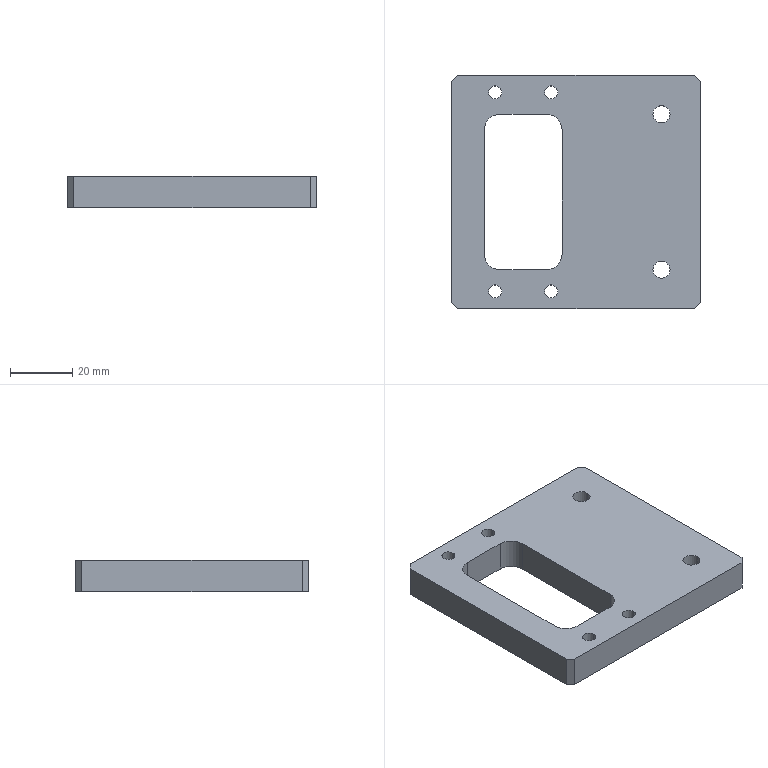Part | SolidWorks | features HoleWzd 2, Chamfer 1, Cut 1, Extrusion 1 | 1 solid | 36 faces | box 80 x 75 x 10 mm | volume 45981 mm3 | cylinder 20 | plane 16 | commonest cylinder face diameters 4.2 x8 10 x8 5.5 x4
STEP:
#1=CARTESIAN_POINT('',(-5.899,32.,5.));
#2=VERTEX_POINT('',#1);
#3=CARTESIAN_POINT('',(-10.099,32.,5.));
#4=VERTEX_POINT('',#3);
#5=CARTESIAN_POINT('',(-7.999,32.,5.));
#6=DIRECTION('',(0.,0.,-1.));
#7=DIRECTION('',(-1.,0.,0.));
#8=AXIS2_PLACEMENT_3D('',#5,#6,#7);
#9=CIRCLE('',#8,2.1);
#10=EDGE_CURVE('',#2,#4,#9,.T.);
#11=ORIENTED_EDGE('',*,*,#10,.F.);
#12=CARTESIAN_POINT('',(-5.899,32.,-5.));
#13=VERTEX_POINT('',#12);
#14=CARTESIAN_POINT('',(-5.899,32.,-5.));
#15=DIRECTION('',(0.,0.,-1.));
#16=VECTOR('',#15,1000.);
#17=LINE('',#14,#16);
#18=EDGE_CURVE('',#2,#13,#17,.T.);
#19=ORIENTED_EDGE('',*,*,#18,.T.);
#20=CARTESIAN_POINT('',(-10.099,32.,-5.));
#21=VERTEX_POINT('',#20);
#22=CARTESIAN_POINT('',(-7.999,32.,-5.));
#23=DIRECTION('',(0.,0.,-1.));
#24=DIRECTION('',(-1.,0.,0.));
#25=AXIS2_PLACEMENT_3D('',#22,#23,#24);
#26=CIRCLE('',#25,2.1);
#27=EDGE_CURVE('',#13,#21,#26,.T.);
#28=ORIENTED_EDGE('',*,*,#27,.T.);
#29=CARTESIAN_POINT('',(-10.099,32.,-5.));
#30=DIRECTION('',(0.,0.,-1.));
#31=VECTOR('',#30,1000.);
#32=LINE('',#29,#31);
#33=EDGE_CURVE('',#4,#21,#32,.T.);
#34=ORIENTED_EDGE('',*,*,#33,.F.);
#35=EDGE_LOOP('',(#11,#19,#28,#34));
#36=FACE_OUTER_BOUND('',#35,.T.);
#37=CARTESIAN_POINT('',(-7.999,32.,-5.));
#38=DIRECTION('',(0.,0.,-1.));
#39=DIRECTION('',(-1.,0.,0.));
#40=AXIS2_PLACEMENT_3D('',#37,#38,#39);
#41=CYLINDRICAL_SURFACE('',#40,2.1);
#42=ADVANCED_FACE('',(#36),#41,.F.);
#43=CARTESIAN_POINT('',(-23.899,32.,5.));
#44=VERTEX_POINT('',#43);
#45=CARTESIAN_POINT('',(-28.099,32.,5.));
#46=VERTEX_POINT('',#45);
#47=CARTESIAN_POINT('',(-25.999,32.,5.));
#48=DIRECTION('',(0.,0.,-1.));
#49=DIRECTION('',(-1.,0.,0.));
#50=AXIS2_PLACEMENT_3D('',#47,#48,#49);
#51=CIRCLE('',#50,2.1);
#52=EDGE_CURVE('',#44,#46,#51,.T.);
#53=ORIENTED_EDGE('',*,*,#52,.F.);
#54=CARTESIAN_POINT('',(-23.899,32.,-5.));
#55=VERTEX_POINT('',#54);
#56=CARTESIAN_POINT('',(-23.899,32.,-5.));
#57=DIRECTION('',(0.,0.,-1.));
#58=VECTOR('',#57,1000.);
#59=LINE('',#56,#58);
#60=EDGE_CURVE('',#44,#55,#59,.T.);
#61=ORIENTED_EDGE('',*,*,#60,.T.);
#62=CARTESIAN_POINT('',(-28.099,32.,-5.));
#63=VERTEX_POINT('',#62);
#64=CARTESIAN_POINT('',(-25.999,32.,-5.));
#65=DIRECTION('',(0.,0.,-1.));
#66=DIRECTION('',(-1.,0.,0.));
#67=AXIS2_PLACEMENT_3D('',#64,#65,#66);
#68=CIRCLE('',#67,2.1);
#69=EDGE_CURVE('',#55,#63,#68,.T.);
#70=ORIENTED_EDGE('',*,*,#69,.T.);
#71=CARTESIAN_POINT('',(-28.099,32.,-5.));
#72=DIRECTION('',(0.,0.,-1.));
#73=VECTOR('',#72,1000.);
#74=LINE('',#71,#73);
#75=EDGE_CURVE('',#46,#63,#74,.T.);
#76=ORIENTED_EDGE('',*,*,#75,.F.);
#77=EDGE_LOOP('',(#53,#61,#70,#76));
#78=FACE_OUTER_BOUND('',#77,.T.);
#79=CARTESIAN_POINT('',(-25.999,32.,-5.));
#80=DIRECTION('',(0.,0.,-1.));
#81=DIRECTION('',(-1.,0.,0.));
#82=AXIS2_PLACEMENT_3D('',#79,#80,#81);
#83=CYLINDRICAL_SURFACE('',#82,2.1);
#84=ADVANCED_FACE('',(#78),#83,.F.);
#85=CARTESIAN_POINT('',(-5.899,-32.,5.));
#86=VERTEX_POINT('',#85);
#87=CARTESIAN_POINT('',(-10.099,-32.,5.));
#88=VERTEX_POINT('',#87);
#89=CARTESIAN_POINT('',(-7.999,-32.,5.));
#90=DIRECTION('',(0.,0.,-1.));
#91=DIRECTION('',(-1.,0.,0.));
#92=AXIS2_PLACEMENT_3D('',#89,#90,#91);
#93=CIRCLE('',#92,2.1);
#94=EDGE_CURVE('',#86,#88,#93,.T.);
#95=ORIENTED_EDGE('',*,*,#94,.F.);
#96=CARTESIAN_POINT('',(-5.899,-32.,-5.));
#97=VERTEX_POINT('',#96);
#98=CARTESIAN_POINT('',(-5.899,-32.,-5.));
#99=DIRECTION('',(0.,0.,-1.));
#100=VECTOR('',#99,1000.);
#101=LINE('',#98,#100);
#102=EDGE_CURVE('',#86,#97,#101,.T.);
#103=ORIENTED_EDGE('',*,*,#102,.T.);
#104=CARTESIAN_POINT('',(-10.099,-32.,-5.));
#105=VERTEX_POINT('',#104);
#106=CARTESIAN_POINT('',(-7.999,-32.,-5.));
#107=DIRECTION('',(0.,0.,-1.));
#108=DIRECTION('',(-1.,0.,0.));
#109=AXIS2_PLACEMENT_3D('',#106,#107,#108);
#110=CIRCLE('',#109,2.1);
#111=EDGE_CURVE('',#97,#105,#110,.T.);
#112=ORIENTED_EDGE('',*,*,#111,.T.);
#113=CARTESIAN_POINT('',(-10.099,-32.,-5.));
#114=DIRECTION('',(0.,0.,-1.));
#115=VECTOR('',#114,1000.);
#116=LINE('',#113,#115);
#117=EDGE_CURVE('',#88,#105,#116,.T.);
#118=ORIENTED_EDGE('',*,*,#117,.F.);
#119=EDGE_LOOP('',(#95,#103,#112,#118));
#120=FACE_OUTER_BOUND('',#119,.T.);
#121=CARTESIAN_POINT('',(-7.999,-32.,-5.));
#122=DIRECTION('',(0.,0.,-1.));
#123=DIRECTION('',(-1.,0.,0.));
#124=AXIS2_PLACEMENT_3D('',#121,#122,#123);
#125=CYLINDRICAL_SURFACE('',#124,2.1);
#126=ADVANCED_FACE('',(#120),#125,.F.);
#127=CARTESIAN_POINT('',(-23.899,-32.,5.));
#128=VERTEX_POINT('',#127);
#129=CARTESIAN_POINT('',(-28.099,-32.,5.));
#130=VERTEX_POINT('',#129);
#131=CARTESIAN_POINT('',(-25.999,-32.,5.));
#132=DIRECTION('',(0.,0.,-1.));
#133=DIRECTION('',(-1.,0.,0.));
#134=AXIS2_PLACEMENT_3D('',#131,#132,#133);
#135=CIRCLE('',#134,2.1);
#136=EDGE_CURVE('',#128,#130,#135,.T.);
#137=ORIENTED_EDGE('',*,*,#136,.F.);
#138=CARTESIAN_POINT('',(-23.899,-32.,-5.));
#139=VERTEX_POINT('',#138);
#140=CARTESIAN_POINT('',(-23.899,-32.,-5.));
#141=DIRECTION('',(0.,0.,-1.));
#142=VECTOR('',#141,1000.);
#143=LINE('',#140,#142);
#144=EDGE_CURVE('',#128,#139,#143,.T.);
#145=ORIENTED_EDGE('',*,*,#144,.T.);
#146=CARTESIAN_POINT('',(-28.099,-32.,-5.));
#147=VERTEX_POINT('',#146);
#148=CARTESIAN_POINT('',(-25.999,-32.,-5.));
#149=DIRECTION('',(0.,0.,-1.));
#150=DIRECTION('',(-1.,0.,0.));
#151=AXIS2_PLACEMENT_3D('',#148,#149,#150);
#152=CIRCLE('',#151,2.1);
#153=EDGE_CURVE('',#139,#147,#152,.T.);
#154=ORIENTED_EDGE('',*,*,#153,.T.);
#155=CARTESIAN_POINT('',(-28.099,-32.,-5.));
#156=DIRECTION('',(0.,0.,-1.));
#157=VECTOR('',#156,1000.);
#158=LINE('',#155,#157);
#159=EDGE_CURVE('',#130,#147,#158,.T.);
#160=ORIENTED_EDGE('',*,*,#159,.F.);
#161=EDGE_LOOP('',(#137,#145,#154,#160));
#162=FACE_OUTER_BOUND('',#161,.T.);
#163=CARTESIAN_POINT('',(-25.999,-32.,-5.));
#164=DIRECTION('',(0.,0.,-1.));
#165=DIRECTION('',(-1.,0.,0.));
#166=AXIS2_PLACEMENT_3D('',#163,#164,#165);
#167=CYLINDRICAL_SURFACE('',#166,2.1);
#168=ADVANCED_FACE('',(#162),#167,.F.);
#169=CARTESIAN_POINT('',(32.5,25.,0.7));
#170=VERTEX_POINT('',#169);
#171=CARTESIAN_POINT('',(22.5,25.,0.7));
#172=VERTEX_POINT('',#171);
#173=CARTESIAN_POINT('',(27.5,25.,0.7));
#174=DIRECTION('',(0.,0.,-1.));
#175=DIRECTION('',(-1.,0.,0.));
#176=AXIS2_PLACEMENT_3D('',#173,#174,#175);
#177=CIRCLE('',#176,5.);
#178=EDGE_CURVE('',#170,#172,#177,.T.);
#179=ORIENTED_EDGE('',*,*,#178,.F.);
#180=CARTESIAN_POINT('',(32.5,25.,-5.));
#181=VERTEX_POINT('',#180);
#182=CARTESIAN_POINT('',(32.5,25.,-5.));
#183=DIRECTION('',(0.,0.,-1.));
#184=VECTOR('',#183,1000.);
#185=LINE('',#182,#184);
#186=EDGE_CURVE('',#170,#181,#185,.T.);
#187=ORIENTED_EDGE('',*,*,#186,.T.);
#188=CARTESIAN_POINT('',(22.5,25.,-5.));
#189=VERTEX_POINT('',#188);
#190=CARTESIAN_POINT('',(27.5,25.,-5.));
#191=DIRECTION('',(0.,0.,-1.));
#192=DIRECTION('',(-1.,0.,0.));
#193=AXIS2_PLACEMENT_3D('',#190,#191,#192);
#194=CIRCLE('',#193,5.);
#195=EDGE_CURVE('',#181,#189,#194,.T.);
#196=ORIENTED_EDGE('',*,*,#195,.T.);
#197=CARTESIAN_POINT('',(22.5,25.,-5.));
#198=DIRECTION('',(0.,0.,-1.));
#199=VECTOR('',#198,1000.);
#200=LINE('',#197,#199);
#201=EDGE_CURVE('',#172,#189,#200,.T.);
#202=ORIENTED_EDGE('',*,*,#201,.F.);
#203=EDGE_LOOP('',(#179,#187,#196,#202));
#204=FACE_OUTER_BOUND('',#203,.T.);
#205=CARTESIAN_POINT('',(27.5,25.,-5.));
#206=DIRECTION('',(0.,0.,-1.));
#207=DIRECTION('',(-1.,0.,0.));
#208=AXIS2_PLACEMENT_3D('',#205,#206,#207);
#209=CYLINDRICAL_SURFACE('',#208,5.);
#210=ADVANCED_FACE('',(#204),#209,.F.);
#211=CARTESIAN_POINT('',(30.25,25.,5.));
#212=VERTEX_POINT('',#211);
#213=CARTESIAN_POINT('',(24.75,25.,5.));
#214=VERTEX_POINT('',#213);
#215=CARTESIAN_POINT('',(27.5,25.,5.));
#216=DIRECTION('',(0.,0.,-1.));
#217=DIRECTION('',(-1.,0.,0.));
#218=AXIS2_PLACEMENT_3D('',#215,#216,#217);
#219=CIRCLE('',#218,2.75);
#220=EDGE_CURVE('',#212,#214,#219,.T.);
#221=ORIENTED_EDGE('',*,*,#220,.F.);
#222=CARTESIAN_POINT('',(30.25,25.,0.7));
#223=VERTEX_POINT('',#222);
#224=CARTESIAN_POINT('',(30.25,25.,-5.));
#225=DIRECTION('',(0.,0.,-1.));
#226=VECTOR('',#225,1000.);
#227=LINE('',#224,#226);
#228=EDGE_CURVE('',#212,#223,#227,.T.);
#229=ORIENTED_EDGE('',*,*,#228,.T.);
#230=CARTESIAN_POINT('',(24.75,25.,0.7));
#231=VERTEX_POINT('',#230);
#232=CARTESIAN_POINT('',(27.5,25.,0.7));
#233=DIRECTION('',(0.,0.,-1.));
#234=DIRECTION('',(-1.,0.,0.));
#235=AXIS2_PLACEMENT_3D('',#232,#233,#234);
#236=CIRCLE('',#235,2.75);
#237=EDGE_CURVE('',#223,#231,#236,.T.);
#238=ORIENTED_EDGE('',*,*,#237,.T.);
#239=CARTESIAN_POINT('',(24.75,25.,-5.));
#240=DIRECTION('',(0.,0.,-1.));
#241=VECTOR('',#240,1000.);
#242=LINE('',#239,#241);
#243=EDGE_CURVE('',#214,#231,#242,.T.);
#244=ORIENTED_EDGE('',*,*,#243,.F.);
#245=EDGE_LOOP('',(#221,#229,#238,#244));
#246=FACE_OUTER_BOUND('',#245,.T.);
#247=CARTESIAN_POINT('',(27.5,25.,-5.));
#248=DIRECTION('',(0.,0.,-1.));
#249=DIRECTION('',(-1.,0.,0.));
#250=AXIS2_PLACEMENT_3D('',#247,#248,#249);
#251=CYLINDRICAL_SURFACE('',#250,2.75);
#252=ADVANCED_FACE('',(#246),#251,.F.);
#253=CARTESIAN_POINT('',(32.5,-25.,0.7));
#254=VERTEX_POINT('',#253);
#255=CARTESIAN_POINT('',(22.5,-25.,0.7));
#256=VERTEX_POINT('',#255);
#257=CARTESIAN_POINT('',(27.5,-25.,0.7));
#258=DIRECTION('',(0.,0.,-1.));
#259=DIRECTION('',(-1.,0.,0.));
#260=AXIS2_PLACEMENT_3D('',#257,#258,#259);
#261=CIRCLE('',#260,5.);
#262=EDGE_CURVE('',#254,#256,#261,.T.);
#263=ORIENTED_EDGE('',*,*,#262,.F.);
#264=CARTESIAN_POINT('',(32.5,-25.,-5.));
#265=VERTEX_POINT('',#264);
#266=CARTESIAN_POINT('',(32.5,-25.,-5.));
#267=DIRECTION('',(0.,0.,-1.));
#268=VECTOR('',#267,1000.);
#269=LINE('',#266,#268);
#270=EDGE_CURVE('',#254,#265,#269,.T.);
#271=ORIENTED_EDGE('',*,*,#270,.T.);
#272=CARTESIAN_POINT('',(22.5,-25.,-5.));
#273=VERTEX_POINT('',#272);
#274=CARTESIAN_POINT('',(27.5,-25.,-5.));
#275=DIRECTION('',(0.,0.,-1.));
#276=DIRECTION('',(-1.,0.,0.));
#277=AXIS2_PLACEMENT_3D('',#274,#275,#276);
#278=CIRCLE('',#277,5.);
#279=EDGE_CURVE('',#265,#273,#278,.T.);
#280=ORIENTED_EDGE('',*,*,#279,.T.);
#281=CARTESIAN_POINT('',(22.5,-25.,-5.));
#282=DIRECTION('',(0.,0.,-1.));
#283=VECTOR('',#282,1000.);
#284=LINE('',#281,#283);
#285=EDGE_CURVE('',#256,#273,#284,.T.);
#286=ORIENTED_EDGE('',*,*,#285,.F.);
#287=EDGE_LOOP('',(#263,#271,#280,#286));
#288=FACE_OUTER_BOUND('',#287,.T.);
#289=CARTESIAN_POINT('',(27.5,-25.,-5.));
#290=DIRECTION('',(0.,0.,-1.));
#291=DIRECTION('',(-1.,0.,0.));
#292=AXIS2_PLACEMENT_3D('',#289,#290,#291);
#293=CYLINDRICAL_SURFACE('',#292,5.);
#294=ADVANCED_FACE('',(#288),#293,.F.);
#295=CARTESIAN_POINT('',(30.25,-25.,5.));
#296=VERTEX_POINT('',#295);
#297=CARTESIAN_POINT('',(24.75,-25.,5.));
#298=VERTEX_POINT('',#297);
#299=CARTESIAN_POINT('',(27.5,-25.,5.));
#300=DIRECTION('',(0.,0.,-1.));
#301=DIRECTION('',(-1.,0.,0.));
#302=AXIS2_PLACEMENT_3D('',#299,#300,#301);
#303=CIRCLE('',#302,2.75);
#304=EDGE_CURVE('',#296,#298,#303,.T.);
#305=ORIENTED_EDGE('',*,*,#304,.F.);
#306=CARTESIAN_POINT('',(30.25,-25.,0.7));
#307=VERTEX_POINT('',#306);
#308=CARTESIAN_POINT('',(30.25,-25.,-5.));
#309=DIRECTION('',(0.,0.,-1.));
#310=VECTOR('',#309,1000.);
#311=LINE('',#308,#310);
#312=EDGE_CURVE('',#296,#307,#311,.T.);
#313=ORIENTED_EDGE('',*,*,#312,.T.);
#314=CARTESIAN_POINT('',(24.75,-25.,0.7));
#315=VERTEX_POINT('',#314);
#316=CARTESIAN_POINT('',(27.5,-25.,0.7));
#317=DIRECTION('',(0.,0.,-1.));
#318=DIRECTION('',(-1.,0.,0.));
#319=AXIS2_PLACEMENT_3D('',#316,#317,#318);
#320=CIRCLE('',#319,2.75);
#321=EDGE_CURVE('',#307,#315,#320,.T.);
#322=ORIENTED_EDGE('',*,*,#321,.T.);
#323=CARTESIAN_POINT('',(24.75,-25.,-5.));
#324=DIRECTION('',(0.,0.,-1.));
#325=VECTOR('',#324,1000.);
#326=LINE('',#323,#325);
#327=EDGE_CURVE('',#298,#315,#326,.T.);
#328=ORIENTED_EDGE('',*,*,#327,.F.);
#329=EDGE_LOOP('',(#305,#313,#322,#328));
#330=FACE_OUTER_BOUND('',#329,.T.);
#331=CARTESIAN_POINT('',(27.5,-25.,-5.));
#332=DIRECTION('',(0.,0.,-1.));
#333=DIRECTION('',(-1.,0.,0.));
#334=AXIS2_PLACEMENT_3D('',#331,#332,#333);
#335=CYLINDRICAL_SURFACE('',#334,2.75);
#336=ADVANCED_FACE('',(#330),#335,.F.);
#337=CARTESIAN_POINT('',(40.,-35.5,5.));
#338=VERTEX_POINT('',#337);
#339=CARTESIAN_POINT('',(40.,35.5,5.));
#340=VERTEX_POINT('',#339);
#341=CARTESIAN_POINT('',(40.,-37.5,5.));
#342=DIRECTION('',(0.,1.,0.));
#343=VECTOR('',#342,1000.);
#344=LINE('',#341,#343);
#345=EDGE_CURVE('',#338,#340,#344,.T.);
#346=ORIENTED_EDGE('',*,*,#345,.F.);
#347=CARTESIAN_POINT('',(40.,-35.5,-5.));
#348=VERTEX_POINT('',#347);
#349=CARTESIAN_POINT('',(40.,-35.5,5.));
#350=DIRECTION('',(0.,0.,-1.));
#351=VECTOR('',#350,1000.);
#352=LINE('',#349,#351);
#353=EDGE_CURVE('',#338,#348,#352,.T.);
#354=ORIENTED_EDGE('',*,*,#353,.T.);
#355=CARTESIAN_POINT('',(40.,35.5,-5.));
#356=VERTEX_POINT('',#355);
#357=CARTESIAN_POINT('',(40.,-37.5,-5.));
#358=DIRECTION('',(0.,1.,0.));
#359=VECTOR('',#358,1000.);
#360=LINE('',#357,#359);
#361=EDGE_CURVE('',#348,#356,#360,.T.);
#362=ORIENTED_EDGE('',*,*,#361,.T.);
#363=CARTESIAN_POINT('',(40.,35.5,5.));
#364=DIRECTION('',(0.,0.,1.));
#365=VECTOR('',#364,1000.);
#366=LINE('',#363,#365);
#367=EDGE_CURVE('',#356,#340,#366,.T.);
#368=ORIENTED_EDGE('',*,*,#367,.T.);
#369=EDGE_LOOP('',(#346,#354,#362,#368));
#370=FACE_OUTER_BOUND('',#369,.T.);
#371=CARTESIAN_POINT('',(40.,-37.5,5.));
#372=DIRECTION('',(-1.,0.,0.));
#373=DIRECTION('',(0.,0.,1.));
#374=AXIS2_PLACEMENT_3D('',#371,#372,#373);
#375=PLANE('',#374);
#376=ADVANCED_FACE('',(#370),#375,.F.);
#377=CARTESIAN_POINT('',(38.,37.5,-5.));
#378=VERTEX_POINT('',#377);
#379=CARTESIAN_POINT('',(-38.,37.5,-5.));
#380=VERTEX_POINT('',#379);
#381=CARTESIAN_POINT('',(-40.,37.5,-5.));
#382=DIRECTION('',(-1.,0.,0.));
#383=VECTOR('',#382,1000.);
#384=LINE('',#381,#383);
#385=EDGE_CURVE('',#378,#380,#384,.T.);
#386=ORIENTED_EDGE('',*,*,#385,.T.);
#387=CARTESIAN_POINT('',(-38.,37.5,5.));
#388=VERTEX_POINT('',#387);
#389=CARTESIAN_POINT('',(-38.,37.5,5.));
#390=DIRECTION('',(0.,0.,1.));
#391=VECTOR('',#390,1000.);
#392=LINE('',#389,#391);
#393=EDGE_CURVE('',#380,#388,#392,.T.);
#394=ORIENTED_EDGE('',*,*,#393,.T.);
#395=CARTESIAN_POINT('',(38.,37.5,5.));
#396=VERTEX_POINT('',#395);
#397=CARTESIAN_POINT('',(-40.,37.5,5.));
#398=DIRECTION('',(-1.,0.,0.));
#399=VECTOR('',#398,1000.);
#400=LINE('',#397,#399);
#401=EDGE_CURVE('',#396,#388,#400,.T.);
#402=ORIENTED_EDGE('',*,*,#401,.F.);
#403=CARTESIAN_POINT('',(38.,37.5,5.));
#404=DIRECTION('',(0.,0.,-1.));
#405=VECTOR('',#404,1000.);
#406=LINE('',#403,#405);
#407=EDGE_CURVE('',#396,#378,#406,.T.);
#408=ORIENTED_EDGE('',*,*,#407,.T.);
#409=EDGE_LOOP('',(#386,#394,#402,#408));
#410=FACE_OUTER_BOUND('',#409,.T.);
#411=CARTESIAN_POINT('',(-40.,37.5,5.));
#412=DIRECTION('',(0.,-1.,0.));
#413=DIRECTION('',(0.,0.,-1.));
#414=AXIS2_PLACEMENT_3D('',#411,#412,#413);
#415=PLANE('',#414);
#416=ADVANCED_FACE('',(#410),#415,.F.);
#417=CARTESIAN_POINT('',(-40.,35.5,-5.));
#418=VERTEX_POINT('',#417);
#419=CARTESIAN_POINT('',(-40.,-35.5,-5.));
#420=VERTEX_POINT('',#419);
#421=CARTESIAN_POINT('',(-40.,-37.5,-5.));
#422=DIRECTION('',(0.,-1.,0.));
#423=VECTOR('',#422,1000.);
#424=LINE('',#421,#423);
#425=EDGE_CURVE('',#418,#420,#424,.T.);
#426=ORIENTED_EDGE('',*,*,#425,.T.);
#427=CARTESIAN_POINT('',(-40.,-35.5,5.));
#428=VERTEX_POINT('',#427);
#429=CARTESIAN_POINT('',(-40.,-35.5,5.));
#430=DIRECTION('',(0.,0.,1.));
#431=VECTOR('',#430,1000.);
#432=LINE('',#429,#431);
#433=EDGE_CURVE('',#420,#428,#432,.T.);
#434=ORIENTED_EDGE('',*,*,#433,.T.);
#435=CARTESIAN_POINT('',(-40.,35.5,5.));
#436=VERTEX_POINT('',#435);
#437=CARTESIAN_POINT('',(-40.,-37.5,5.));
#438=DIRECTION('',(0.,-1.,0.));
#439=VECTOR('',#438,1000.);
#440=LINE('',#437,#439);
#441=EDGE_CURVE('',#436,#428,#440,.T.);
#442=ORIENTED_EDGE('',*,*,#441,.F.);
#443=CARTESIAN_POINT('',(-40.,35.5,5.));
#444=DIRECTION('',(0.,0.,-1.));
#445=VECTOR('',#444,1000.);
#446=LINE('',#443,#445);
#447=EDGE_CURVE('',#436,#418,#446,.T.);
#448=ORIENTED_EDGE('',*,*,#447,.T.);
#449=EDGE_LOOP('',(#426,#434,#442,#448));
#450=FACE_OUTER_BOUND('',#449,.T.);
#451=CARTESIAN_POINT('',(-40.,-37.5,5.));
#452=DIRECTION('',(1.,0.,0.));
#453=DIRECTION('',(0.,0.,-1.));
#454=AXIS2_PLACEMENT_3D('',#451,#452,#453);
#455=PLANE('',#454);
#456=ADVANCED_FACE('',(#450),#455,.F.);
#457=CARTESIAN_POINT('',(-38.,-37.5,-5.));
#458=VERTEX_POINT('',#457);
#459=CARTESIAN_POINT('',(38.,-37.5,-5.));
#460=VERTEX_POINT('',#459);
#461=CARTESIAN_POINT('',(-40.,-37.5,-5.));
#462=DIRECTION('',(1.,0.,0.));
#463=VECTOR('',#462,1000.);
#464=LINE('',#461,#463);
#465=EDGE_CURVE('',#458,#460,#464,.T.);
#466=ORIENTED_EDGE('',*,*,#465,.T.);
#467=CARTESIAN_POINT('',(38.,-37.5,5.));
#468=VERTEX_POINT('',#467);
#469=CARTESIAN_POINT('',(38.,-37.5,5.));
#470=DIRECTION('',(0.,0.,1.));
#471=VECTOR('',#470,1000.);
#472=LINE('',#469,#471);
#473=EDGE_CURVE('',#460,#468,#472,.T.);
#474=ORIENTED_EDGE('',*,*,#473,.T.);
#475=CARTESIAN_POINT('',(-38.,-37.5,5.));
#476=VERTEX_POINT('',#475);
#477=CARTESIAN_POINT('',(-40.,-37.5,5.));
#478=DIRECTION('',(1.,0.,0.));
#479=VECTOR('',#478,1000.);
#480=LINE('',#477,#479);
#481=EDGE_CURVE('',#476,#468,#480,.T.);
#482=ORIENTED_EDGE('',*,*,#481,.F.);
#483=CARTESIAN_POINT('',(-38.,-37.5,5.));
#484=DIRECTION('',(0.,0.,-1.));
#485=VECTOR('',#484,1000.);
#486=LINE('',#483,#485);
#487=EDGE_CURVE('',#476,#458,#486,.T.);
#488=ORIENTED_EDGE('',*,*,#487,.T.);
#489=EDGE_LOOP('',(#466,#474,#482,#488));
#490=FACE_OUTER_BOUND('',#489,.T.);
#491=CARTESIAN_POINT('',(-40.,-37.5,5.));
#492=DIRECTION('',(0.,1.,0.));
#493=DIRECTION('',(0.,0.,1.));
#494=AXIS2_PLACEMENT_3D('',#491,#492,#493);
#495=PLANE('',#494);
#496=ADVANCED_FACE('',(#490),#495,.F.);
#497=CARTESIAN_POINT('',(-9.499,-25.,5.));
#498=VERTEX_POINT('',#497);
#499=CARTESIAN_POINT('',(-24.499,-25.,5.));
#500=VERTEX_POINT('',#499);
#501=CARTESIAN_POINT('',(-9.499,-25.,5.));
#502=DIRECTION('',(-1.,0.,0.));
#503=VECTOR('',#502,1000.);
#504=LINE('',#501,#503);
#505=EDGE_CURVE('',#498,#500,#504,.T.);
#506=ORIENTED_EDGE('',*,*,#505,.T.);
#507=CARTESIAN_POINT('',(-29.499,-20.,5.));
#508=VERTEX_POINT('',#507);
#509=CARTESIAN_POINT('',(-24.499,-20.,5.));
#510=DIRECTION('',(0.,0.,-1.));
#511=DIRECTION('',(-1.,0.,0.));
#512=AXIS2_PLACEMENT_3D('',#509,#510,#511);
#513=CIRCLE('',#512,5.);
#514=EDGE_CURVE('',#500,#508,#513,.T.);
#515=ORIENTED_EDGE('',*,*,#514,.T.);
#516=CARTESIAN_POINT('',(-29.499,20.,5.));
#517=VERTEX_POINT('',#516);
#518=CARTESIAN_POINT('',(-29.499,-20.,5.));
#519=DIRECTION('',(0.,1.,0.));
#520=VECTOR('',#519,1000.);
#521=LINE('',#518,#520);
#522=EDGE_CURVE('',#508,#517,#521,.T.);
#523=ORIENTED_EDGE('',*,*,#522,.T.);
#524=CARTESIAN_POINT('',(-24.499,25.,5.));
#525=VERTEX_POINT('',#524);
#526=CARTESIAN_POINT('',(-24.499,20.,5.));
#527=DIRECTION('',(0.,0.,-1.));
#528=DIRECTION('',(1.,0.,0.));
#529=AXIS2_PLACEMENT_3D('',#526,#527,#528);
#530=CIRCLE('',#529,5.);
#531=EDGE_CURVE('',#517,#525,#530,.T.);
#532=ORIENTED_EDGE('',*,*,#531,.T.);
#533=CARTESIAN_POINT('',(-9.499,25.,5.));
#534=VERTEX_POINT('',#533);
#535=CARTESIAN_POINT('',(-9.499,25.,5.));
#536=DIRECTION('',(1.,0.,0.));
#537=VECTOR('',#536,1000.);
#538=LINE('',#535,#537);
#539=EDGE_CURVE('',#525,#534,#538,.T.);
#540=ORIENTED_EDGE('',*,*,#539,.T.);
#541=CARTESIAN_POINT('',(-4.499,20.,5.));
#542=VERTEX_POINT('',#541);
#543=CARTESIAN_POINT('',(-9.499,20.,5.));
#544=DIRECTION('',(0.,0.,-1.));
#545=DIRECTION('',(1.,0.,0.));
#546=AXIS2_PLACEMENT_3D('',#543,#544,#545);
#547=CIRCLE('',#546,5.);
#548=EDGE_CURVE('',#534,#542,#547,.T.);
#549=ORIENTED_EDGE('',*,*,#548,.T.);
#550=CARTESIAN_POINT('',(-4.499,-20.,5.));
#551=VERTEX_POINT('',#550);
#552=CARTESIAN_POINT('',(-4.499,-20.,5.));
#553=DIRECTION('',(0.,-1.,0.));
#554=VECTOR('',#553,1000.);
#555=LINE('',#552,#554);
#556=EDGE_CURVE('',#542,#551,#555,.T.);
#557=ORIENTED_EDGE('',*,*,#556,.T.);
#558=CARTESIAN_POINT('',(-9.499,-20.,5.));
#559=DIRECTION('',(0.,0.,-1.));
#560=DIRECTION('',(1.,0.,0.));
#561=AXIS2_PLACEMENT_3D('',#558,#559,#560);
#562=CIRCLE('',#561,5.);
#563=EDGE_CURVE('',#551,#498,#562,.T.);
#564=ORIENTED_EDGE('',*,*,#563,.T.);
#565=EDGE_LOOP('',(#506,#515,#523,#532,#540,#549,#557,#564));
#566=FACE_BOUND('',#565,.T.);
#567=CARTESIAN_POINT('',(-7.999,32.,5.));
#568=DIRECTION('',(0.,0.,-1.));
#569=DIRECTION('',(-1.,0.,0.));
#570=AXIS2_PLACEMENT_3D('',#567,#568,#569);
#571=CIRCLE('',#570,2.1);
#572=EDGE_CURVE('',#4,#2,#571,.T.);
#573=ORIENTED_EDGE('',*,*,#572,.T.);
#574=ORIENTED_EDGE('',*,*,#10,.T.);
#575=EDGE_LOOP('',(#573,#574));
#576=FACE_BOUND('',#575,.T.);
#577=CARTESIAN_POINT('',(-25.999,32.,5.));
#578=DIRECTION('',(0.,0.,-1.));
#579=DIRECTION('',(-1.,0.,0.));
#580=AXIS2_PLACEMENT_3D('',#577,#578,#579);
#581=CIRCLE('',#580,2.1);
#582=EDGE_CURVE('',#46,#44,#581,.T.);
#583=ORIENTED_EDGE('',*,*,#582,.T.);
#584=ORIENTED_EDGE('',*,*,#52,.T.);
#585=EDGE_LOOP('',(#583,#584));
#586=FACE_BOUND('',#585,.T.);
#587=CARTESIAN_POINT('',(-7.999,-32.,5.));
#588=DIRECTION('',(0.,0.,-1.));
#589=DIRECTION('',(-1.,0.,0.));
#590=AXIS2_PLACEMENT_3D('',#587,#588,#589);
#591=CIRCLE('',#590,2.1);
#592=EDGE_CURVE('',#88,#86,#591,.T.);
#593=ORIENTED_EDGE('',*,*,#592,.T.);
#594=ORIENTED_EDGE('',*,*,#94,.T.);
#595=EDGE_LOOP('',(#593,#594));
#596=FACE_BOUND('',#595,.T.);
#597=CARTESIAN_POINT('',(-25.999,-32.,5.));
#598=DIRECTION('',(0.,0.,-1.));
#599=DIRECTION('',(-1.,0.,0.));
#600=AXIS2_PLACEMENT_3D('',#597,#598,#599);
#601=CIRCLE('',#600,2.1);
#602=EDGE_CURVE('',#130,#128,#601,.T.);
#603=ORIENTED_EDGE('',*,*,#602,.T.);
#604=ORIENTED_EDGE('',*,*,#136,.T.);
#605=EDGE_LOOP('',(#603,#604));
#606=FACE_BOUND('',#605,.T.);
#607=CARTESIAN_POINT('',(27.5,25.,5.));
#608=DIRECTION('',(0.,0.,-1.));
#609=DIRECTION('',(-1.,0.,0.));
#610=AXIS2_PLACEMENT_3D('',#607,#608,#609);
#611=CIRCLE('',#610,2.75);
#612=EDGE_CURVE('',#214,#212,#611,.T.);
#613=ORIENTED_EDGE('',*,*,#612,.T.);
#614=ORIENTED_EDGE('',*,*,#220,.T.);
#615=EDGE_LOOP('',(#613,#614));
#616=FACE_BOUND('',#615,.T.);
#617=CARTESIAN_POINT('',(27.5,-25.,5.));
#618=DIRECTION('',(0.,0.,-1.));
#619=DIRECTION('',(-1.,0.,0.));
#620=AXIS2_PLACEMENT_3D('',#617,#618,#619);
#621=CIRCLE('',#620,2.75);
#622=EDGE_CURVE('',#298,#296,#621,.T.);
#623=ORIENTED_EDGE('',*,*,#622,.T.);
#624=ORIENTED_EDGE('',*,*,#304,.T.);
#625=EDGE_LOOP('',(#623,#624));
#626=FACE_BOUND('',#625,.T.);
#627=ORIENTED_EDGE('',*,*,#481,.T.);
#628=CARTESIAN_POINT('',(40.,-35.5,5.));
#629=DIRECTION('',(0.7071,0.7071,0.));
#630=VECTOR('',#629,1000.);
#631=LINE('',#628,#630);
#632=EDGE_CURVE('',#468,#338,#631,.T.);
#633=ORIENTED_EDGE('',*,*,#632,.T.);
#634=ORIENTED_EDGE('',*,*,#345,.T.);
#635=CARTESIAN_POINT('',(38.,37.5,5.));
#636=DIRECTION('',(-0.7071,0.7071,0.));
#637=VECTOR('',#636,1000.);
#638=LINE('',#635,#637);
#639=EDGE_CURVE('',#340,#396,#638,.T.);
#640=ORIENTED_EDGE('',*,*,#639,.T.);
#641=ORIENTED_EDGE('',*,*,#401,.T.);
#642=CARTESIAN_POINT('',(-40.,35.5,5.));
#643=DIRECTION('',(-0.7071,-0.7071,0.));
#644=VECTOR('',#643,1000.);
#645=LINE('',#642,#644);
#646=EDGE_CURVE('',#388,#436,#645,.T.);
#647=ORIENTED_EDGE('',*,*,#646,.T.);
#648=ORIENTED_EDGE('',*,*,#441,.T.);
#649=CARTESIAN_POINT('',(-38.,-37.5,5.));
#650=DIRECTION('',(0.7071,-0.7071,0.));
#651=VECTOR('',#650,1000.);
#652=LINE('',#649,#651);
#653=EDGE_CURVE('',#428,#476,#652,.T.);
#654=ORIENTED_EDGE('',*,*,#653,.T.);
#655=EDGE_LOOP('',(#627,#633,#634,#640,#641,#647,#648,#654));
#656=FACE_OUTER_BOUND('',#655,.T.);
#657=CARTESIAN_POINT('',(0.,0.,5.));
#658=DIRECTION('',(0.,0.,-1.));
#659=DIRECTION('',(-1.,0.,0.));
#660=AXIS2_PLACEMENT_3D('',#657,#658,#659);
#661=PLANE('',#660);
#662=ADVANCED_FACE('',(#566,#576,#586,#596,#606,#616,#626,#656),#661,.F.);
#663=CARTESIAN_POINT('',(-24.499,-25.,-5.));
#664=VERTEX_POINT('',#663);
#665=CARTESIAN_POINT('',(-29.499,-20.,-5.));
#666=VERTEX_POINT('',#665);
#667=CARTESIAN_POINT('',(-24.499,-20.,-5.));
#668=DIRECTION('',(0.,0.,-1.));
#669=DIRECTION('',(-1.,0.,0.));
#670=AXIS2_PLACEMENT_3D('',#667,#668,#669);
#671=CIRCLE('',#670,5.);
#672=EDGE_CURVE('',#664,#666,#671,.T.);
#673=ORIENTED_EDGE('',*,*,#672,.F.);
#674=CARTESIAN_POINT('',(-9.499,-25.,-5.));
#675=VERTEX_POINT('',#674);
#676=CARTESIAN_POINT('',(-9.499,-25.,-5.));
#677=DIRECTION('',(-1.,0.,0.));
#678=VECTOR('',#677,1000.);
#679=LINE('',#676,#678);
#680=EDGE_CURVE('',#675,#664,#679,.T.);
#681=ORIENTED_EDGE('',*,*,#680,.F.);
#682=CARTESIAN_POINT('',(-4.499,-20.,-5.));
#683=VERTEX_POINT('',#682);
#684=CARTESIAN_POINT('',(-9.499,-20.,-5.));
#685=DIRECTION('',(0.,0.,-1.));
#686=DIRECTION('',(1.,0.,0.));
#687=AXIS2_PLACEMENT_3D('',#684,#685,#686);
#688=CIRCLE('',#687,5.);
#689=EDGE_CURVE('',#683,#675,#688,.T.);
#690=ORIENTED_EDGE('',*,*,#689,.F.);
#691=CARTESIAN_POINT('',(-4.499,20.,-5.));
#692=VERTEX_POINT('',#691);
#693=CARTESIAN_POINT('',(-4.499,-20.,-5.));
#694=DIRECTION('',(0.,-1.,0.));
#695=VECTOR('',#694,1000.);
#696=LINE('',#693,#695);
#697=EDGE_CURVE('',#692,#683,#696,.T.);
#698=ORIENTED_EDGE('',*,*,#697,.F.);
#699=CARTESIAN_POINT('',(-9.499,25.,-5.));
#700=VERTEX_POINT('',#699);
#701=CARTESIAN_POINT('',(-9.499,20.,-5.));
#702=DIRECTION('',(0.,0.,-1.));
#703=DIRECTION('',(1.,0.,0.));
#704=AXIS2_PLACEMENT_3D('',#701,#702,#703);
#705=CIRCLE('',#704,5.);
#706=EDGE_CURVE('',#700,#692,#705,.T.);
#707=ORIENTED_EDGE('',*,*,#706,.F.);
#708=CARTESIAN_POINT('',(-24.499,25.,-5.));
#709=VERTEX_POINT('',#708);
#710=CARTESIAN_POINT('',(-9.499,25.,-5.));
#711=DIRECTION('',(1.,0.,0.));
#712=VECTOR('',#711,1000.);
#713=LINE('',#710,#712);
#714=EDGE_CURVE('',#709,#700,#713,.T.);
#715=ORIENTED_EDGE('',*,*,#714,.F.);
#716=CARTESIAN_POINT('',(-29.499,20.,-5.));
#717=VERTEX_POINT('',#716);
#718=CARTESIAN_POINT('',(-24.499,20.,-5.));
#719=DIRECTION('',(0.,0.,-1.));
#720=DIRECTION('',(1.,0.,0.));
#721=AXIS2_PLACEMENT_3D('',#718,#719,#720);
#722=CIRCLE('',#721,5.);
#723=EDGE_CURVE('',#717,#709,#722,.T.);
#724=ORIENTED_EDGE('',*,*,#723,.F.);
#725=CARTESIAN_POINT('',(-29.499,-20.,-5.));
#726=DIRECTION('',(0.,1.,0.));
#727=VECTOR('',#726,1000.);
#728=LINE('',#725,#727);
#729=EDGE_CURVE('',#666,#717,#728,.T.);
#730=ORIENTED_EDGE('',*,*,#729,.F.);
#731=EDGE_LOOP('',(#673,#681,#690,#698,#707,#715,#724,#730));
#732=FACE_BOUND('',#731,.T.);
#733=CARTESIAN_POINT('',(-7.999,32.,-5.));
#734=DIRECTION('',(0.,0.,-1.));
#735=DIRECTION('',(-1.,0.,0.));
#736=AXIS2_PLACEMENT_3D('',#733,#734,#735);
#737=CIRCLE('',#736,2.1);
#738=EDGE_CURVE('',#21,#13,#737,.T.);
#739=ORIENTED_EDGE('',*,*,#738,.F.);
#740=ORIENTED_EDGE('',*,*,#27,.F.);
#741=EDGE_LOOP('',(#739,#740));
#742=FACE_BOUND('',#741,.T.);
#743=CARTESIAN_POINT('',(-25.999,32.,-5.));
#744=DIRECTION('',(0.,0.,-1.));
#745=DIRECTION('',(-1.,0.,0.));
#746=AXIS2_PLACEMENT_3D('',#743,#744,#745);
#747=CIRCLE('',#746,2.1);
#748=EDGE_CURVE('',#63,#55,#747,.T.);
#749=ORIENTED_EDGE('',*,*,#748,.F.);
#750=ORIENTED_EDGE('',*,*,#69,.F.);
#751=EDGE_LOOP('',(#749,#750));
#752=FACE_BOUND('',#751,.T.);
#753=CARTESIAN_POINT('',(-7.999,-32.,-5.));
#754=DIRECTION('',(0.,0.,-1.));
#755=DIRECTION('',(-1.,0.,0.));
#756=AXIS2_PLACEMENT_3D('',#753,#754,#755);
#757=CIRCLE('',#756,2.1);
#758=EDGE_CURVE('',#105,#97,#757,.T.);
#759=ORIENTED_EDGE('',*,*,#758,.F.);
#760=ORIENTED_EDGE('',*,*,#111,.F.);
#761=EDGE_LOOP('',(#759,#760));
#762=FACE_BOUND('',#761,.T.);
#763=CARTESIAN_POINT('',(-25.999,-32.,-5.));
#764=DIRECTION('',(0.,0.,-1.));
#765=DIRECTION('',(-1.,0.,0.));
#766=AXIS2_PLACEMENT_3D('',#763,#764,#765);
#767=CIRCLE('',#766,2.1);
#768=EDGE_CURVE('',#147,#139,#767,.T.);
#769=ORIENTED_EDGE('',*,*,#768,.F.);
#770=ORIENTED_EDGE('',*,*,#153,.F.);
#771=EDGE_LOOP('',(#769,#770));
#772=FACE_BOUND('',#771,.T.);
#773=CARTESIAN_POINT('',(27.5,25.,-5.));
#774=DIRECTION('',(0.,0.,-1.));
#775=DIRECTION('',(-1.,0.,0.));
#776=AXIS2_PLACEMENT_3D('',#773,#774,#775);
#777=CIRCLE('',#776,5.);
#778=EDGE_CURVE('',#189,#181,#777,.T.);
#779=ORIENTED_EDGE('',*,*,#778,.F.);
#780=ORIENTED_EDGE('',*,*,#195,.F.);
#781=EDGE_LOOP('',(#779,#780));
#782=FACE_BOUND('',#781,.T.);
#783=CARTESIAN_POINT('',(27.5,-25.,-5.));
#784=DIRECTION('',(0.,0.,-1.));
#785=DIRECTION('',(-1.,0.,0.));
#786=AXIS2_PLACEMENT_3D('',#783,#784,#785);
#787=CIRCLE('',#786,5.);
#788=EDGE_CURVE('',#273,#265,#787,.T.);
#789=ORIENTED_EDGE('',*,*,#788,.F.);
#790=ORIENTED_EDGE('',*,*,#279,.F.);
#791=EDGE_LOOP('',(#789,#790));
#792=FACE_BOUND('',#791,.T.);
#793=ORIENTED_EDGE('',*,*,#361,.F.);
#794=CARTESIAN_POINT('',(37.75,-37.75,-5.));
#795=DIRECTION('',(-0.7071,-0.7071,0.));
#796=VECTOR('',#795,1000.);
#797=LINE('',#794,#796);
#798=EDGE_CURVE('',#348,#460,#797,.T.);
#799=ORIENTED_EDGE('',*,*,#798,.T.);
#800=ORIENTED_EDGE('',*,*,#465,.F.);
#801=CARTESIAN_POINT('',(-37.75,-37.75,-5.));
#802=DIRECTION('',(-0.7071,0.7071,0.));
#803=VECTOR('',#802,1000.);
#804=LINE('',#801,#803);
#805=EDGE_CURVE('',#458,#420,#804,.T.);
#806=ORIENTED_EDGE('',*,*,#805,.T.);
#807=ORIENTED_EDGE('',*,*,#425,.F.);
#808=CARTESIAN_POINT('',(-37.75,37.75,-5.));
#809=DIRECTION('',(0.7071,0.7071,0.));
#810=VECTOR('',#809,1000.);
#811=LINE('',#808,#810);
#812=EDGE_CURVE('',#418,#380,#811,.T.);
#813=ORIENTED_EDGE('',*,*,#812,.T.);
#814=ORIENTED_EDGE('',*,*,#385,.F.);
#815=CARTESIAN_POINT('',(37.75,37.75,-5.));
#816=DIRECTION('',(0.7071,-0.7071,0.));
#817=VECTOR('',#816,1000.);
#818=LINE('',#815,#817);
#819=EDGE_CURVE('',#378,#356,#818,.T.);
#820=ORIENTED_EDGE('',*,*,#819,.T.);
#821=EDGE_LOOP('',(#793,#799,#800,#806,#807,#813,#814,#820));
#822=FACE_OUTER_BOUND('',#821,.T.);
#823=CARTESIAN_POINT('',(0.,0.,-5.));
#824=DIRECTION('',(0.,0.,-1.));
#825=DIRECTION('',(-1.,0.,0.));
#826=AXIS2_PLACEMENT_3D('',#823,#824,#825);
#827=PLANE('',#826);
#828=ADVANCED_FACE('',(#732,#742,#752,#762,#772,#782,#792,#822),#827,.T.);
#829=ORIENTED_EDGE('',*,*,#632,.F.);
#830=ORIENTED_EDGE('',*,*,#473,.F.);
#831=ORIENTED_EDGE('',*,*,#798,.F.);
#832=ORIENTED_EDGE('',*,*,#353,.F.);
#833=EDGE_LOOP('',(#829,#830,#831,#832));
#834=FACE_OUTER_BOUND('',#833,.T.);
#835=CARTESIAN_POINT('',(40.,-35.5,5.));
#836=DIRECTION('',(-0.7071,0.7071,0.));
#837=DIRECTION('',(0.,0.,-1.));
#838=AXIS2_PLACEMENT_3D('',#835,#836,#837);
#839=PLANE('',#838);
#840=ADVANCED_FACE('',(#834),#839,.F.);
#841=ORIENTED_EDGE('',*,*,#653,.F.);
#842=ORIENTED_EDGE('',*,*,#433,.F.);
#843=ORIENTED_EDGE('',*,*,#805,.F.);
#844=ORIENTED_EDGE('',*,*,#487,.F.);
#845=EDGE_LOOP('',(#841,#842,#843,#844));
#846=FACE_OUTER_BOUND('',#845,.T.);
#847=CARTESIAN_POINT('',(-38.,-37.5,5.));
#848=DIRECTION('',(0.7071,0.7071,0.));
#849=DIRECTION('',(0.,0.,-1.));
#850=AXIS2_PLACEMENT_3D('',#847,#848,#849);
#851=PLANE('',#850);
#852=ADVANCED_FACE('',(#846),#851,.F.);
#853=ORIENTED_EDGE('',*,*,#646,.F.);
#854=ORIENTED_EDGE('',*,*,#393,.F.);
#855=ORIENTED_EDGE('',*,*,#812,.F.);
#856=ORIENTED_EDGE('',*,*,#447,.F.);
#857=EDGE_LOOP('',(#853,#854,#855,#856));
#858=FACE_OUTER_BOUND('',#857,.T.);
#859=CARTESIAN_POINT('',(-40.,35.5,5.));
#860=DIRECTION('',(0.7071,-0.7071,0.));
#861=DIRECTION('',(0.,0.,-1.));
#862=AXIS2_PLACEMENT_3D('',#859,#860,#861);
#863=PLANE('',#862);
#864=ADVANCED_FACE('',(#858),#863,.F.);
#865=ORIENTED_EDGE('',*,*,#639,.F.);
#866=ORIENTED_EDGE('',*,*,#367,.F.);
#867=ORIENTED_EDGE('',*,*,#819,.F.);
#868=ORIENTED_EDGE('',*,*,#407,.F.);
#869=EDGE_LOOP('',(#865,#866,#867,#868));
#870=FACE_OUTER_BOUND('',#869,.T.);
#871=CARTESIAN_POINT('',(38.,37.5,5.));
#872=DIRECTION('',(-0.7071,-0.7071,0.));
#873=DIRECTION('',(0.,0.,-1.));
#874=AXIS2_PLACEMENT_3D('',#871,#872,#873);
#875=PLANE('',#874);
#876=ADVANCED_FACE('',(#870),#875,.F.);
#877=ORIENTED_EDGE('',*,*,#312,.F.);
#878=ORIENTED_EDGE('',*,*,#622,.F.);
#879=ORIENTED_EDGE('',*,*,#327,.T.);
#880=CARTESIAN_POINT('',(27.5,-25.,0.7));
#881=DIRECTION('',(0.,0.,-1.));
#882=DIRECTION('',(-1.,0.,0.));
#883=AXIS2_PLACEMENT_3D('',#880,#881,#882);
#884=CIRCLE('',#883,2.75);
#885=EDGE_CURVE('',#315,#307,#884,.T.);
#886=ORIENTED_EDGE('',*,*,#885,.T.);
#887=EDGE_LOOP('',(#877,#878,#879,#886));
#888=FACE_OUTER_BOUND('',#887,.T.);
#889=CARTESIAN_POINT('',(27.5,-25.,-5.));
#890=DIRECTION('',(0.,0.,-1.));
#891=DIRECTION('',(-1.,0.,0.));
#892=AXIS2_PLACEMENT_3D('',#889,#890,#891);
#893=CYLINDRICAL_SURFACE('',#892,2.75);
#894=ADVANCED_FACE('',(#888),#893,.F.);
#895=ORIENTED_EDGE('',*,*,#885,.F.);
#896=ORIENTED_EDGE('',*,*,#321,.F.);
#897=EDGE_LOOP('',(#895,#896));
#898=FACE_BOUND('',#897,.T.);
#899=CARTESIAN_POINT('',(27.5,-25.,0.7));
#900=DIRECTION('',(0.,0.,-1.));
#901=DIRECTION('',(-1.,0.,0.));
#902=AXIS2_PLACEMENT_3D('',#899,#900,#901);
#903=CIRCLE('',#902,5.);
#904=EDGE_CURVE('',#256,#254,#903,.T.);
#905=ORIENTED_EDGE('',*,*,#904,.T.);
#906=ORIENTED_EDGE('',*,*,#262,.T.);
#907=EDGE_LOOP('',(#905,#906));
#908=FACE_OUTER_BOUND('',#907,.T.);
#909=CARTESIAN_POINT('',(30.25,-25.,0.7));
#910=DIRECTION('',(0.,0.,1.));
#911=DIRECTION('',(1.,0.,0.));
#912=AXIS2_PLACEMENT_3D('',#909,#910,#911);
#913=PLANE('',#912);
#914=ADVANCED_FACE('',(#898,#908),#913,.F.);
#915=ORIENTED_EDGE('',*,*,#270,.F.);
#916=ORIENTED_EDGE('',*,*,#904,.F.);
#917=ORIENTED_EDGE('',*,*,#285,.T.);
#918=ORIENTED_EDGE('',*,*,#788,.T.);
#919=EDGE_LOOP('',(#915,#916,#917,#918));
#920=FACE_OUTER_BOUND('',#919,.T.);
#921=CARTESIAN_POINT('',(27.5,-25.,-5.));
#922=DIRECTION('',(0.,0.,-1.));
#923=DIRECTION('',(-1.,0.,0.));
#924=AXIS2_PLACEMENT_3D('',#921,#922,#923);
#925=CYLINDRICAL_SURFACE('',#924,5.);
#926=ADVANCED_FACE('',(#920),#925,.F.);
#927=ORIENTED_EDGE('',*,*,#228,.F.);
#928=ORIENTED_EDGE('',*,*,#612,.F.);
#929=ORIENTED_EDGE('',*,*,#243,.T.);
#930=CARTESIAN_POINT('',(27.5,25.,0.7));
#931=DIRECTION('',(0.,0.,-1.));
#932=DIRECTION('',(-1.,0.,0.));
#933=AXIS2_PLACEMENT_3D('',#930,#931,#932);
#934=CIRCLE('',#933,2.75);
#935=EDGE_CURVE('',#231,#223,#934,.T.);
#936=ORIENTED_EDGE('',*,*,#935,.T.);
#937=EDGE_LOOP('',(#927,#928,#929,#936));
#938=FACE_OUTER_BOUND('',#937,.T.);
#939=CARTESIAN_POINT('',(27.5,25.,-5.));
#940=DIRECTION('',(0.,0.,-1.));
#941=DIRECTION('',(-1.,0.,0.));
#942=AXIS2_PLACEMENT_3D('',#939,#940,#941);
#943=CYLINDRICAL_SURFACE('',#942,2.75);
#944=ADVANCED_FACE('',(#938),#943,.F.);
#945=ORIENTED_EDGE('',*,*,#935,.F.);
#946=ORIENTED_EDGE('',*,*,#237,.F.);
#947=EDGE_LOOP('',(#945,#946));
#948=FACE_BOUND('',#947,.T.);
#949=CARTESIAN_POINT('',(27.5,25.,0.7));
#950=DIRECTION('',(0.,0.,-1.));
#951=DIRECTION('',(-1.,0.,0.));
#952=AXIS2_PLACEMENT_3D('',#949,#950,#951);
#953=CIRCLE('',#952,5.);
#954=EDGE_CURVE('',#172,#170,#953,.T.);
#955=ORIENTED_EDGE('',*,*,#954,.T.);
#956=ORIENTED_EDGE('',*,*,#178,.T.);
#957=EDGE_LOOP('',(#955,#956));
#958=FACE_OUTER_BOUND('',#957,.T.);
#959=CARTESIAN_POINT('',(30.25,25.,0.7));
#960=DIRECTION('',(0.,0.,1.));
#961=DIRECTION('',(1.,0.,0.));
#962=AXIS2_PLACEMENT_3D('',#959,#960,#961);
#963=PLANE('',#962);
#964=ADVANCED_FACE('',(#948,#958),#963,.F.);
#965=ORIENTED_EDGE('',*,*,#186,.F.);
#966=ORIENTED_EDGE('',*,*,#954,.F.);
#967=ORIENTED_EDGE('',*,*,#201,.T.);
#968=ORIENTED_EDGE('',*,*,#778,.T.);
#969=EDGE_LOOP('',(#965,#966,#967,#968));
#970=FACE_OUTER_BOUND('',#969,.T.);
#971=CARTESIAN_POINT('',(27.5,25.,-5.));
#972=DIRECTION('',(0.,0.,-1.));
#973=DIRECTION('',(-1.,0.,0.));
#974=AXIS2_PLACEMENT_3D('',#971,#972,#973);
#975=CYLINDRICAL_SURFACE('',#974,5.);
#976=ADVANCED_FACE('',(#970),#975,.F.);
#977=ORIENTED_EDGE('',*,*,#144,.F.);
#978=ORIENTED_EDGE('',*,*,#602,.F.);
#979=ORIENTED_EDGE('',*,*,#159,.T.);
#980=ORIENTED_EDGE('',*,*,#768,.T.);
#981=EDGE_LOOP('',(#977,#978,#979,#980));
#982=FACE_OUTER_BOUND('',#981,.T.);
#983=CARTESIAN_POINT('',(-25.999,-32.,-5.));
#984=DIRECTION('',(0.,0.,-1.));
#985=DIRECTION('',(-1.,0.,0.));
#986=AXIS2_PLACEMENT_3D('',#983,#984,#985);
#987=CYLINDRICAL_SURFACE('',#986,2.1);
#988=ADVANCED_FACE('',(#982),#987,.F.);
#989=ORIENTED_EDGE('',*,*,#102,.F.);
#990=ORIENTED_EDGE('',*,*,#592,.F.);
#991=ORIENTED_EDGE('',*,*,#117,.T.);
#992=ORIENTED_EDGE('',*,*,#758,.T.);
#993=EDGE_LOOP('',(#989,#990,#991,#992));
#994=FACE_OUTER_BOUND('',#993,.T.);
#995=CARTESIAN_POINT('',(-7.999,-32.,-5.));
#996=DIRECTION('',(0.,0.,-1.));
#997=DIRECTION('',(-1.,0.,0.));
#998=AXIS2_PLACEMENT_3D('',#995,#996,#997);
#999=CYLINDRICAL_SURFACE('',#998,2.1);
#1000=ADVANCED_FACE('',(#994),#999,.F.);
#1001=ORIENTED_EDGE('',*,*,#60,.F.);
#1002=ORIENTED_EDGE('',*,*,#582,.F.);
#1003=ORIENTED_EDGE('',*,*,#75,.T.);
#1004=ORIENTED_EDGE('',*,*,#748,.T.);
#1005=EDGE_LOOP('',(#1001,#1002,#1003,#1004));
#1006=FACE_OUTER_BOUND('',#1005,.T.);
#1007=CARTESIAN_POINT('',(-25.999,32.,-5.));
#1008=DIRECTION('',(0.,0.,-1.));
#1009=DIRECTION('',(-1.,0.,0.));
#1010=AXIS2_PLACEMENT_3D('',#1007,#1008,#1009);
#1011=CYLINDRICAL_SURFACE('',#1010,2.1);
#1012=ADVANCED_FACE('',(#1006),#1011,.F.);
#1013=ORIENTED_EDGE('',*,*,#18,.F.);
#1014=ORIENTED_EDGE('',*,*,#572,.F.);
#1015=ORIENTED_EDGE('',*,*,#33,.T.);
#1016=ORIENTED_EDGE('',*,*,#738,.T.);
#1017=EDGE_LOOP('',(#1013,#1014,#1015,#1016));
#1018=FACE_OUTER_BOUND('',#1017,.T.);
#1019=CARTESIAN_POINT('',(-7.999,32.,-5.));
#1020=DIRECTION('',(0.,0.,-1.));
#1021=DIRECTION('',(-1.,0.,0.));
#1022=AXIS2_PLACEMENT_3D('',#1019,#1020,#1021);
#1023=CYLINDRICAL_SURFACE('',#1022,2.1);
#1024=ADVANCED_FACE('',(#1018),#1023,.F.);
#1025=ORIENTED_EDGE('',*,*,#672,.T.);
#1026=CARTESIAN_POINT('',(-29.499,-20.,5.));
#1027=DIRECTION('',(0.,0.,-1.));
#1028=VECTOR('',#1027,1000.);
#1029=LINE('',#1026,#1028);
#1030=EDGE_CURVE('',#508,#666,#1029,.T.);
#1031=ORIENTED_EDGE('',*,*,#1030,.F.);
#1032=ORIENTED_EDGE('',*,*,#514,.F.);
#1033=CARTESIAN_POINT('',(-24.499,-25.,5.));
#1034=DIRECTION('',(0.,0.,-1.));
#1035=VECTOR('',#1034,1000.);
#1036=LINE('',#1033,#1035);
#1037=EDGE_CURVE('',#500,#664,#1036,.T.);
#1038=ORIENTED_EDGE('',*,*,#1037,.T.);
#1039=EDGE_LOOP('',(#1025,#1031,#1032,#1038));
#1040=FACE_OUTER_BOUND('',#1039,.T.);
#1041=CARTESIAN_POINT('',(-24.499,-20.,5.));
#1042=DIRECTION('',(0.,0.,-1.));
#1043=DIRECTION('',(-1.,0.,0.));
#1044=AXIS2_PLACEMENT_3D('',#1041,#1042,#1043);
#1045=CYLINDRICAL_SURFACE('',#1044,5.);
#1046=ADVANCED_FACE('',(#1040),#1045,.F.);
#1047=ORIENTED_EDGE('',*,*,#680,.T.);
#1048=ORIENTED_EDGE('',*,*,#1037,.F.);
#1049=ORIENTED_EDGE('',*,*,#505,.F.);
#1050=CARTESIAN_POINT('',(-9.499,-25.,5.));
#1051=DIRECTION('',(0.,0.,-1.));
#1052=VECTOR('',#1051,1000.);
#1053=LINE('',#1050,#1052);
#1054=EDGE_CURVE('',#498,#675,#1053,.T.);
#1055=ORIENTED_EDGE('',*,*,#1054,.T.);
#1056=EDGE_LOOP('',(#1047,#1048,#1049,#1055));
#1057=FACE_OUTER_BOUND('',#1056,.T.);
#1058=CARTESIAN_POINT('',(-9.499,-25.,5.));
#1059=DIRECTION('',(0.,-1.,0.));
#1060=DIRECTION('',(0.,0.,-1.));
#1061=AXIS2_PLACEMENT_3D('',#1058,#1059,#1060);
#1062=PLANE('',#1061);
#1063=ADVANCED_FACE('',(#1057),#1062,.F.);
#1064=ORIENTED_EDGE('',*,*,#689,.T.);
#1065=ORIENTED_EDGE('',*,*,#1054,.F.);
#1066=ORIENTED_EDGE('',*,*,#563,.F.);
#1067=CARTESIAN_POINT('',(-4.499,-20.,5.));
#1068=DIRECTION('',(0.,0.,-1.));
#1069=VECTOR('',#1068,1000.);
#1070=LINE('',#1067,#1069);
#1071=EDGE_CURVE('',#551,#683,#1070,.T.);
#1072=ORIENTED_EDGE('',*,*,#1071,.T.);
#1073=EDGE_LOOP('',(#1064,#1065,#1066,#1072));
#1074=FACE_OUTER_BOUND('',#1073,.T.);
#1075=CARTESIAN_POINT('',(-9.499,-20.,5.));
#1076=DIRECTION('',(0.,0.,-1.));
#1077=DIRECTION('',(-1.,0.,0.));
#1078=AXIS2_PLACEMENT_3D('',#1075,#1076,#1077);
#1079=CYLINDRICAL_SURFACE('',#1078,5.);
#1080=ADVANCED_FACE('',(#1074),#1079,.F.);
#1081=ORIENTED_EDGE('',*,*,#697,.T.);
#1082=ORIENTED_EDGE('',*,*,#1071,.F.);
#1083=ORIENTED_EDGE('',*,*,#556,.F.);
#1084=CARTESIAN_POINT('',(-4.499,20.,5.));
#1085=DIRECTION('',(0.,0.,-1.));
#1086=VECTOR('',#1085,1000.);
#1087=LINE('',#1084,#1086);
#1088=EDGE_CURVE('',#542,#692,#1087,.T.);
#1089=ORIENTED_EDGE('',*,*,#1088,.T.);
#1090=EDGE_LOOP('',(#1081,#1082,#1083,#1089));
#1091=FACE_OUTER_BOUND('',#1090,.T.);
#1092=CARTESIAN_POINT('',(-4.499,-20.,5.));
#1093=DIRECTION('',(1.,0.,0.));
#1094=DIRECTION('',(0.,0.,-1.));
#1095=AXIS2_PLACEMENT_3D('',#1092,#1093,#1094);
#1096=PLANE('',#1095);
#1097=ADVANCED_FACE('',(#1091),#1096,.F.);
#1098=ORIENTED_EDGE('',*,*,#706,.T.);
#1099=ORIENTED_EDGE('',*,*,#1088,.F.);
#1100=ORIENTED_EDGE('',*,*,#548,.F.);
#1101=CARTESIAN_POINT('',(-9.499,25.,5.));
#1102=DIRECTION('',(0.,0.,-1.));
#1103=VECTOR('',#1102,1000.);
#1104=LINE('',#1101,#1103);
#1105=EDGE_CURVE('',#534,#700,#1104,.T.);
#1106=ORIENTED_EDGE('',*,*,#1105,.T.);
#1107=EDGE_LOOP('',(#1098,#1099,#1100,#1106));
#1108=FACE_OUTER_BOUND('',#1107,.T.);
#1109=CARTESIAN_POINT('',(-9.499,20.,5.));
#1110=DIRECTION('',(0.,0.,-1.));
#1111=DIRECTION('',(-1.,0.,0.));
#1112=AXIS2_PLACEMENT_3D('',#1109,#1110,#1111);
#1113=CYLINDRICAL_SURFACE('',#1112,5.);
#1114=ADVANCED_FACE('',(#1108),#1113,.F.);
#1115=ORIENTED_EDGE('',*,*,#714,.T.);
#1116=ORIENTED_EDGE('',*,*,#1105,.F.);
#1117=ORIENTED_EDGE('',*,*,#539,.F.);
#1118=CARTESIAN_POINT('',(-24.499,25.,5.));
#1119=DIRECTION('',(0.,0.,-1.));
#1120=VECTOR('',#1119,1000.);
#1121=LINE('',#1118,#1120);
#1122=EDGE_CURVE('',#525,#709,#1121,.T.);
#1123=ORIENTED_EDGE('',*,*,#1122,.T.);
#1124=EDGE_LOOP('',(#1115,#1116,#1117,#1123));
#1125=FACE_OUTER_BOUND('',#1124,.T.);
#1126=CARTESIAN_POINT('',(-9.499,25.,5.));
#1127=DIRECTION('',(0.,1.,0.));
#1128=DIRECTION('',(0.,0.,1.));
#1129=AXIS2_PLACEMENT_3D('',#1126,#1127,#1128);
#1130=PLANE('',#1129);
#1131=ADVANCED_FACE('',(#1125),#1130,.F.);
#1132=ORIENTED_EDGE('',*,*,#723,.T.);
#1133=ORIENTED_EDGE('',*,*,#1122,.F.);
#1134=ORIENTED_EDGE('',*,*,#531,.F.);
#1135=CARTESIAN_POINT('',(-29.499,20.,5.));
#1136=DIRECTION('',(0.,0.,-1.));
#1137=VECTOR('',#1136,1000.);
#1138=LINE('',#1135,#1137);
#1139=EDGE_CURVE('',#517,#717,#1138,.T.);
#1140=ORIENTED_EDGE('',*,*,#1139,.T.);
#1141=EDGE_LOOP('',(#1132,#1133,#1134,#1140));
#1142=FACE_OUTER_BOUND('',#1141,.T.);
#1143=CARTESIAN_POINT('',(-24.499,20.,5.));
#1144=DIRECTION('',(0.,0.,-1.));
#1145=DIRECTION('',(-1.,0.,0.));
#1146=AXIS2_PLACEMENT_3D('',#1143,#1144,#1145);
#1147=CYLINDRICAL_SURFACE('',#1146,5.);
#1148=ADVANCED_FACE('',(#1142),#1147,.F.);
#1149=ORIENTED_EDGE('',*,*,#729,.T.);
#1150=ORIENTED_EDGE('',*,*,#1139,.F.);
#1151=ORIENTED_EDGE('',*,*,#522,.F.);
#1152=ORIENTED_EDGE('',*,*,#1030,.T.);
#1153=EDGE_LOOP('',(#1149,#1150,#1151,#1152));
#1154=FACE_OUTER_BOUND('',#1153,.T.);
#1155=CARTESIAN_POINT('',(-29.499,-20.,5.));
#1156=DIRECTION('',(-1.,0.,0.));
#1157=DIRECTION('',(0.,0.,1.));
#1158=AXIS2_PLACEMENT_3D('',#1155,#1156,#1157);
#1159=PLANE('',#1158);
#1160=ADVANCED_FACE('',(#1154),#1159,.F.);
#1161=CLOSED_SHELL('',(#42,#84,#126,#168,#210,#252,#294,#336,#376,#416,#456,#496,#662,#828,#840,#852,#864,#876,#894,#914,#926,#944,#964,#976,#988,#1000,#1012,#1024,#1046,#1063,#1080,#1097,#1114,#1131,#1148,#1160));
#1162=MANIFOLD_SOLID_BREP('',#1161);
#1163=CARTESIAN_POINT('',(0.,0.,0.));
#1164=DIRECTION('',(0.,0.,1.));
#1165=DIRECTION('',(1.,0.,0.));
#1166=AXIS2_PLACEMENT_3D('',#1163,#1164,#1165);
#1167=(LENGTH_UNIT()NAMED_UNIT(*)SI_UNIT(.MILLI.,.METRE.));
#1168=UNCERTAINTY_MEASURE_WITH_UNIT(LENGTH_MEASURE(0.00001),#1167,'','');
#1169=(NAMED_UNIT(*)PLANE_ANGLE_UNIT()SI_UNIT($,.RADIAN.));
#1170=(NAMED_UNIT(*)SI_UNIT($,.STERADIAN.)SOLID_ANGLE_UNIT());
#1171=(GEOMETRIC_REPRESENTATION_CONTEXT(3)GLOBAL_UNCERTAINTY_ASSIGNED_CONTEXT((#1168))GLOBAL_UNIT_ASSIGNED_CONTEXT((#1167,#1169,#1170))REPRESENTATION_CONTEXT('',''));
#1172=ADVANCED_BREP_SHAPE_REPRESENTATION('',(#1162,#1166),#1171);